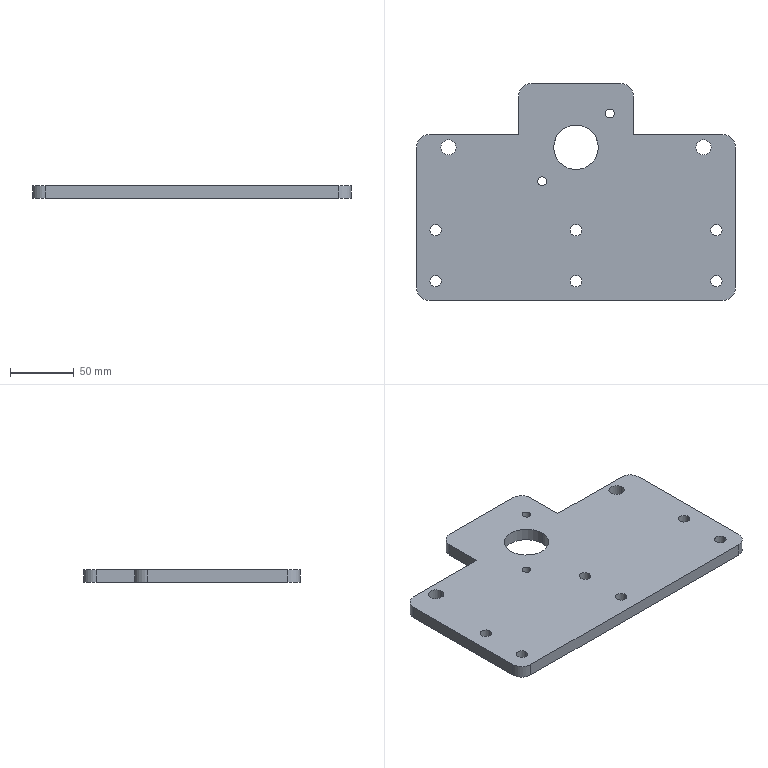Part | SolidWorks | features HoleWzd 3, ICE 2, Extrusion 1, Fillet 1, LPattern 1, MirrorPattern 1 | 1 solid | 38 faces | box 250 x 170 x 10 mm | volume 343286 mm3 | cylinder 28 | plane 10 | commonest cylinder face diameters 9 x12 20 x6 6.8 x4 12 x4 35 x2
STEP:
#1=CARTESIAN_POINT('',(-29.915,8.485,-5.));
#2=VERTEX_POINT('',#1);
#3=CARTESIAN_POINT('',(-23.115,8.485,-5.));
#4=VERTEX_POINT('',#3);
#5=CARTESIAN_POINT('',(-26.515,8.485,-5.));
#6=DIRECTION('',(0.,0.,1.));
#7=DIRECTION('',(1.,0.,0.));
#8=AXIS2_PLACEMENT_3D('',#5,#6,#7);
#9=CIRCLE('',#8,3.4);
#10=EDGE_CURVE('',#2,#4,#9,.T.);
#11=ORIENTED_EDGE('',*,*,#10,.F.);
#12=CARTESIAN_POINT('',(-29.915,8.485,5.));
#13=VERTEX_POINT('',#12);
#14=CARTESIAN_POINT('',(-29.915,8.485,5.));
#15=DIRECTION('',(0.,0.,1.));
#16=VECTOR('',#15,1000.);
#17=LINE('',#14,#16);
#18=EDGE_CURVE('',#2,#13,#17,.T.);
#19=ORIENTED_EDGE('',*,*,#18,.T.);
#20=CARTESIAN_POINT('',(-23.115,8.485,5.));
#21=VERTEX_POINT('',#20);
#22=CARTESIAN_POINT('',(-26.515,8.485,5.));
#23=DIRECTION('',(0.,0.,1.));
#24=DIRECTION('',(1.,0.,0.));
#25=AXIS2_PLACEMENT_3D('',#22,#23,#24);
#26=CIRCLE('',#25,3.4);
#27=EDGE_CURVE('',#13,#21,#26,.T.);
#28=ORIENTED_EDGE('',*,*,#27,.T.);
#29=CARTESIAN_POINT('',(-23.115,8.485,5.));
#30=DIRECTION('',(0.,0.,1.));
#31=VECTOR('',#30,1000.);
#32=LINE('',#29,#31);
#33=EDGE_CURVE('',#4,#21,#32,.T.);
#34=ORIENTED_EDGE('',*,*,#33,.F.);
#35=EDGE_LOOP('',(#11,#19,#28,#34));
#36=FACE_OUTER_BOUND('',#35,.T.);
#37=CARTESIAN_POINT('',(-26.515,8.485,5.));
#38=DIRECTION('',(0.,0.,1.));
#39=DIRECTION('',(1.,0.,0.));
#40=AXIS2_PLACEMENT_3D('',#37,#38,#39);
#41=CYLINDRICAL_SURFACE('',#40,3.4);
#42=ADVANCED_FACE('',(#36),#41,.F.);
#43=CARTESIAN_POINT('',(23.115,61.515,-5.));
#44=VERTEX_POINT('',#43);
#45=CARTESIAN_POINT('',(29.915,61.515,-5.));
#46=VERTEX_POINT('',#45);
#47=CARTESIAN_POINT('',(26.515,61.515,-5.));
#48=DIRECTION('',(0.,0.,1.));
#49=DIRECTION('',(1.,0.,0.));
#50=AXIS2_PLACEMENT_3D('',#47,#48,#49);
#51=CIRCLE('',#50,3.4);
#52=EDGE_CURVE('',#44,#46,#51,.T.);
#53=ORIENTED_EDGE('',*,*,#52,.F.);
#54=CARTESIAN_POINT('',(23.115,61.515,5.));
#55=VERTEX_POINT('',#54);
#56=CARTESIAN_POINT('',(23.115,61.515,5.));
#57=DIRECTION('',(0.,0.,1.));
#58=VECTOR('',#57,1000.);
#59=LINE('',#56,#58);
#60=EDGE_CURVE('',#44,#55,#59,.T.);
#61=ORIENTED_EDGE('',*,*,#60,.T.);
#62=CARTESIAN_POINT('',(29.915,61.515,5.));
#63=VERTEX_POINT('',#62);
#64=CARTESIAN_POINT('',(26.515,61.515,5.));
#65=DIRECTION('',(0.,0.,1.));
#66=DIRECTION('',(1.,0.,0.));
#67=AXIS2_PLACEMENT_3D('',#64,#65,#66);
#68=CIRCLE('',#67,3.4);
#69=EDGE_CURVE('',#55,#63,#68,.T.);
#70=ORIENTED_EDGE('',*,*,#69,.T.);
#71=CARTESIAN_POINT('',(29.915,61.515,5.));
#72=DIRECTION('',(0.,0.,1.));
#73=VECTOR('',#72,1000.);
#74=LINE('',#71,#73);
#75=EDGE_CURVE('',#46,#63,#74,.T.);
#76=ORIENTED_EDGE('',*,*,#75,.F.);
#77=EDGE_LOOP('',(#53,#61,#70,#76));
#78=FACE_OUTER_BOUND('',#77,.T.);
#79=CARTESIAN_POINT('',(26.515,61.515,5.));
#80=DIRECTION('',(0.,0.,1.));
#81=DIRECTION('',(1.,0.,0.));
#82=AXIS2_PLACEMENT_3D('',#79,#80,#81);
#83=CYLINDRICAL_SURFACE('',#82,3.4);
#84=ADVANCED_FACE('',(#78),#83,.F.);
#85=CARTESIAN_POINT('',(-17.5,35.,-5.));
#86=VERTEX_POINT('',#85);
#87=CARTESIAN_POINT('',(17.5,35.,-5.));
#88=VERTEX_POINT('',#87);
#89=CARTESIAN_POINT('',(0.,35.,-5.));
#90=DIRECTION('',(0.,0.,1.));
#91=DIRECTION('',(1.,0.,0.));
#92=AXIS2_PLACEMENT_3D('',#89,#90,#91);
#93=CIRCLE('',#92,17.5);
#94=EDGE_CURVE('',#86,#88,#93,.T.);
#95=ORIENTED_EDGE('',*,*,#94,.F.);
#96=CARTESIAN_POINT('',(-17.5,35.,5.));
#97=VERTEX_POINT('',#96);
#98=CARTESIAN_POINT('',(-17.5,35.,-5.));
#99=DIRECTION('',(0.,0.,1.));
#100=VECTOR('',#99,1000.);
#101=LINE('',#98,#100);
#102=EDGE_CURVE('',#86,#97,#101,.T.);
#103=ORIENTED_EDGE('',*,*,#102,.T.);
#104=CARTESIAN_POINT('',(17.5,35.,5.));
#105=VERTEX_POINT('',#104);
#106=CARTESIAN_POINT('',(0.,35.,5.));
#107=DIRECTION('',(0.,0.,1.));
#108=DIRECTION('',(1.,0.,0.));
#109=AXIS2_PLACEMENT_3D('',#106,#107,#108);
#110=CIRCLE('',#109,17.5);
#111=EDGE_CURVE('',#97,#105,#110,.T.);
#112=ORIENTED_EDGE('',*,*,#111,.T.);
#113=CARTESIAN_POINT('',(17.5,35.,-5.));
#114=DIRECTION('',(0.,0.,1.));
#115=VECTOR('',#114,1000.);
#116=LINE('',#113,#115);
#117=EDGE_CURVE('',#88,#105,#116,.T.);
#118=ORIENTED_EDGE('',*,*,#117,.F.);
#119=EDGE_LOOP('',(#95,#103,#112,#118));
#120=FACE_OUTER_BOUND('',#119,.T.);
#121=CARTESIAN_POINT('',(0.,35.,-5.));
#122=DIRECTION('',(0.,0.,1.));
#123=DIRECTION('',(1.,0.,0.));
#124=AXIS2_PLACEMENT_3D('',#121,#122,#123);
#125=CYLINDRICAL_SURFACE('',#124,17.5);
#126=ADVANCED_FACE('',(#120),#125,.F.);
#127=CARTESIAN_POINT('',(-106.,35.,-5.));
#128=VERTEX_POINT('',#127);
#129=CARTESIAN_POINT('',(-94.,35.,-5.));
#130=VERTEX_POINT('',#129);
#131=CARTESIAN_POINT('',(-100.,35.,-5.));
#132=DIRECTION('',(0.,0.,1.));
#133=DIRECTION('',(1.,0.,0.));
#134=AXIS2_PLACEMENT_3D('',#131,#132,#133);
#135=CIRCLE('',#134,6.);
#136=EDGE_CURVE('',#128,#130,#135,.T.);
#137=ORIENTED_EDGE('',*,*,#136,.F.);
#138=CARTESIAN_POINT('',(-106.,35.,5.));
#139=VERTEX_POINT('',#138);
#140=CARTESIAN_POINT('',(-106.,35.,5.));
#141=DIRECTION('',(0.,0.,1.));
#142=VECTOR('',#141,1000.);
#143=LINE('',#140,#142);
#144=EDGE_CURVE('',#128,#139,#143,.T.);
#145=ORIENTED_EDGE('',*,*,#144,.T.);
#146=CARTESIAN_POINT('',(-94.,35.,5.));
#147=VERTEX_POINT('',#146);
#148=CARTESIAN_POINT('',(-100.,35.,5.));
#149=DIRECTION('',(0.,0.,1.));
#150=DIRECTION('',(1.,0.,0.));
#151=AXIS2_PLACEMENT_3D('',#148,#149,#150);
#152=CIRCLE('',#151,6.);
#153=EDGE_CURVE('',#139,#147,#152,.T.);
#154=ORIENTED_EDGE('',*,*,#153,.T.);
#155=CARTESIAN_POINT('',(-94.,35.,5.));
#156=DIRECTION('',(0.,0.,1.));
#157=VECTOR('',#156,1000.);
#158=LINE('',#155,#157);
#159=EDGE_CURVE('',#130,#147,#158,.T.);
#160=ORIENTED_EDGE('',*,*,#159,.F.);
#161=EDGE_LOOP('',(#137,#145,#154,#160));
#162=FACE_OUTER_BOUND('',#161,.T.);
#163=CARTESIAN_POINT('',(-100.,35.,5.));
#164=DIRECTION('',(0.,0.,1.));
#165=DIRECTION('',(1.,0.,0.));
#166=AXIS2_PLACEMENT_3D('',#163,#164,#165);
#167=CYLINDRICAL_SURFACE('',#166,6.);
#168=ADVANCED_FACE('',(#162),#167,.F.);
#169=CARTESIAN_POINT('',(94.,35.,-5.));
#170=VERTEX_POINT('',#169);
#171=CARTESIAN_POINT('',(106.,35.,-5.));
#172=VERTEX_POINT('',#171);
#173=CARTESIAN_POINT('',(100.,35.,-5.));
#174=DIRECTION('',(0.,0.,1.));
#175=DIRECTION('',(1.,0.,0.));
#176=AXIS2_PLACEMENT_3D('',#173,#174,#175);
#177=CIRCLE('',#176,6.);
#178=EDGE_CURVE('',#170,#172,#177,.T.);
#179=ORIENTED_EDGE('',*,*,#178,.F.);
#180=CARTESIAN_POINT('',(94.,35.,5.));
#181=VERTEX_POINT('',#180);
#182=CARTESIAN_POINT('',(94.,35.,5.));
#183=DIRECTION('',(0.,0.,1.));
#184=VECTOR('',#183,1000.);
#185=LINE('',#182,#184);
#186=EDGE_CURVE('',#170,#181,#185,.T.);
#187=ORIENTED_EDGE('',*,*,#186,.T.);
#188=CARTESIAN_POINT('',(106.,35.,5.));
#189=VERTEX_POINT('',#188);
#190=CARTESIAN_POINT('',(100.,35.,5.));
#191=DIRECTION('',(0.,0.,1.));
#192=DIRECTION('',(1.,0.,0.));
#193=AXIS2_PLACEMENT_3D('',#190,#191,#192);
#194=CIRCLE('',#193,6.);
#195=EDGE_CURVE('',#181,#189,#194,.T.);
#196=ORIENTED_EDGE('',*,*,#195,.T.);
#197=CARTESIAN_POINT('',(106.,35.,5.));
#198=DIRECTION('',(0.,0.,1.));
#199=VECTOR('',#198,1000.);
#200=LINE('',#197,#199);
#201=EDGE_CURVE('',#172,#189,#200,.T.);
#202=ORIENTED_EDGE('',*,*,#201,.F.);
#203=EDGE_LOOP('',(#179,#187,#196,#202));
#204=FACE_OUTER_BOUND('',#203,.T.);
#205=CARTESIAN_POINT('',(100.,35.,5.));
#206=DIRECTION('',(0.,0.,1.));
#207=DIRECTION('',(1.,0.,0.));
#208=AXIS2_PLACEMENT_3D('',#205,#206,#207);
#209=CYLINDRICAL_SURFACE('',#208,6.);
#210=ADVANCED_FACE('',(#204),#209,.F.);
#211=CARTESIAN_POINT('',(105.5,-70.,-5.));
#212=VERTEX_POINT('',#211);
#213=CARTESIAN_POINT('',(114.5,-70.,-5.));
#214=VERTEX_POINT('',#213);
#215=CARTESIAN_POINT('',(110.,-70.,-5.));
#216=DIRECTION('',(0.,0.,1.));
#217=DIRECTION('',(1.,0.,0.));
#218=AXIS2_PLACEMENT_3D('',#215,#216,#217);
#219=CIRCLE('',#218,4.5);
#220=EDGE_CURVE('',#212,#214,#219,.T.);
#221=ORIENTED_EDGE('',*,*,#220,.F.);
#222=CARTESIAN_POINT('',(105.5,-70.,5.));
#223=VERTEX_POINT('',#222);
#224=CARTESIAN_POINT('',(105.5,-70.,5.));
#225=DIRECTION('',(0.,0.,1.));
#226=VECTOR('',#225,1000.);
#227=LINE('',#224,#226);
#228=EDGE_CURVE('',#212,#223,#227,.T.);
#229=ORIENTED_EDGE('',*,*,#228,.T.);
#230=CARTESIAN_POINT('',(114.5,-70.,5.));
#231=VERTEX_POINT('',#230);
#232=CARTESIAN_POINT('',(110.,-70.,5.));
#233=DIRECTION('',(0.,0.,1.));
#234=DIRECTION('',(1.,0.,0.));
#235=AXIS2_PLACEMENT_3D('',#232,#233,#234);
#236=CIRCLE('',#235,4.5);
#237=EDGE_CURVE('',#223,#231,#236,.T.);
#238=ORIENTED_EDGE('',*,*,#237,.T.);
#239=CARTESIAN_POINT('',(114.5,-70.,5.));
#240=DIRECTION('',(0.,0.,1.));
#241=VECTOR('',#240,1000.);
#242=LINE('',#239,#241);
#243=EDGE_CURVE('',#214,#231,#242,.T.);
#244=ORIENTED_EDGE('',*,*,#243,.F.);
#245=EDGE_LOOP('',(#221,#229,#238,#244));
#246=FACE_OUTER_BOUND('',#245,.T.);
#247=CARTESIAN_POINT('',(110.,-70.,5.));
#248=DIRECTION('',(0.,0.,1.));
#249=DIRECTION('',(1.,0.,0.));
#250=AXIS2_PLACEMENT_3D('',#247,#248,#249);
#251=CYLINDRICAL_SURFACE('',#250,4.5);
#252=ADVANCED_FACE('',(#246),#251,.F.);
#253=CARTESIAN_POINT('',(-4.5,-70.,-5.));
#254=VERTEX_POINT('',#253);
#255=CARTESIAN_POINT('',(4.5,-70.,-5.));
#256=VERTEX_POINT('',#255);
#257=CARTESIAN_POINT('',(0.,-70.,-5.));
#258=DIRECTION('',(0.,0.,1.));
#259=DIRECTION('',(1.,0.,0.));
#260=AXIS2_PLACEMENT_3D('',#257,#258,#259);
#261=CIRCLE('',#260,4.5);
#262=EDGE_CURVE('',#254,#256,#261,.T.);
#263=ORIENTED_EDGE('',*,*,#262,.F.);
#264=CARTESIAN_POINT('',(-4.5,-70.,5.));
#265=VERTEX_POINT('',#264);
#266=CARTESIAN_POINT('',(-4.5,-70.,5.));
#267=DIRECTION('',(0.,0.,1.));
#268=VECTOR('',#267,1000.);
#269=LINE('',#266,#268);
#270=EDGE_CURVE('',#254,#265,#269,.T.);
#271=ORIENTED_EDGE('',*,*,#270,.T.);
#272=CARTESIAN_POINT('',(4.5,-70.,5.));
#273=VERTEX_POINT('',#272);
#274=CARTESIAN_POINT('',(0.,-70.,5.));
#275=DIRECTION('',(0.,0.,1.));
#276=DIRECTION('',(1.,0.,0.));
#277=AXIS2_PLACEMENT_3D('',#274,#275,#276);
#278=CIRCLE('',#277,4.5);
#279=EDGE_CURVE('',#265,#273,#278,.T.);
#280=ORIENTED_EDGE('',*,*,#279,.T.);
#281=CARTESIAN_POINT('',(4.5,-70.,5.));
#282=DIRECTION('',(0.,0.,1.));
#283=VECTOR('',#282,1000.);
#284=LINE('',#281,#283);
#285=EDGE_CURVE('',#256,#273,#284,.T.);
#286=ORIENTED_EDGE('',*,*,#285,.F.);
#287=EDGE_LOOP('',(#263,#271,#280,#286));
#288=FACE_OUTER_BOUND('',#287,.T.);
#289=CARTESIAN_POINT('',(0.,-70.,5.));
#290=DIRECTION('',(0.,0.,1.));
#291=DIRECTION('',(1.,0.,0.));
#292=AXIS2_PLACEMENT_3D('',#289,#290,#291);
#293=CYLINDRICAL_SURFACE('',#292,4.5);
#294=ADVANCED_FACE('',(#288),#293,.F.);
#295=CARTESIAN_POINT('',(105.5,-30.,-5.));
#296=VERTEX_POINT('',#295);
#297=CARTESIAN_POINT('',(114.5,-30.,-5.));
#298=VERTEX_POINT('',#297);
#299=CARTESIAN_POINT('',(110.,-30.,-5.));
#300=DIRECTION('',(0.,0.,1.));
#301=DIRECTION('',(1.,0.,0.));
#302=AXIS2_PLACEMENT_3D('',#299,#300,#301);
#303=CIRCLE('',#302,4.5);
#304=EDGE_CURVE('',#296,#298,#303,.T.);
#305=ORIENTED_EDGE('',*,*,#304,.F.);
#306=CARTESIAN_POINT('',(105.5,-30.,5.));
#307=VERTEX_POINT('',#306);
#308=CARTESIAN_POINT('',(105.5,-30.,5.));
#309=DIRECTION('',(0.,0.,1.));
#310=VECTOR('',#309,1000.);
#311=LINE('',#308,#310);
#312=EDGE_CURVE('',#296,#307,#311,.T.);
#313=ORIENTED_EDGE('',*,*,#312,.T.);
#314=CARTESIAN_POINT('',(114.5,-30.,5.));
#315=VERTEX_POINT('',#314);
#316=CARTESIAN_POINT('',(110.,-30.,5.));
#317=DIRECTION('',(0.,0.,1.));
#318=DIRECTION('',(1.,0.,0.));
#319=AXIS2_PLACEMENT_3D('',#316,#317,#318);
#320=CIRCLE('',#319,4.5);
#321=EDGE_CURVE('',#307,#315,#320,.T.);
#322=ORIENTED_EDGE('',*,*,#321,.T.);
#323=CARTESIAN_POINT('',(114.5,-30.,5.));
#324=DIRECTION('',(0.,0.,1.));
#325=VECTOR('',#324,1000.);
#326=LINE('',#323,#325);
#327=EDGE_CURVE('',#298,#315,#326,.T.);
#328=ORIENTED_EDGE('',*,*,#327,.F.);
#329=EDGE_LOOP('',(#305,#313,#322,#328));
#330=FACE_OUTER_BOUND('',#329,.T.);
#331=CARTESIAN_POINT('',(110.,-30.,5.));
#332=DIRECTION('',(0.,0.,1.));
#333=DIRECTION('',(1.,0.,0.));
#334=AXIS2_PLACEMENT_3D('',#331,#332,#333);
#335=CYLINDRICAL_SURFACE('',#334,4.5);
#336=ADVANCED_FACE('',(#330),#335,.F.);
#337=CARTESIAN_POINT('',(-4.5,-30.,-5.));
#338=VERTEX_POINT('',#337);
#339=CARTESIAN_POINT('',(4.5,-30.,-5.));
#340=VERTEX_POINT('',#339);
#341=CARTESIAN_POINT('',(0.,-30.,-5.));
#342=DIRECTION('',(0.,0.,1.));
#343=DIRECTION('',(1.,0.,0.));
#344=AXIS2_PLACEMENT_3D('',#341,#342,#343);
#345=CIRCLE('',#344,4.5);
#346=EDGE_CURVE('',#338,#340,#345,.T.);
#347=ORIENTED_EDGE('',*,*,#346,.F.);
#348=CARTESIAN_POINT('',(-4.5,-30.,5.));
#349=VERTEX_POINT('',#348);
#350=CARTESIAN_POINT('',(-4.5,-30.,5.));
#351=DIRECTION('',(0.,0.,1.));
#352=VECTOR('',#351,1000.);
#353=LINE('',#350,#352);
#354=EDGE_CURVE('',#338,#349,#353,.T.);
#355=ORIENTED_EDGE('',*,*,#354,.T.);
#356=CARTESIAN_POINT('',(4.5,-30.,5.));
#357=VERTEX_POINT('',#356);
#358=CARTESIAN_POINT('',(0.,-30.,5.));
#359=DIRECTION('',(0.,0.,1.));
#360=DIRECTION('',(1.,0.,0.));
#361=AXIS2_PLACEMENT_3D('',#358,#359,#360);
#362=CIRCLE('',#361,4.5);
#363=EDGE_CURVE('',#349,#357,#362,.T.);
#364=ORIENTED_EDGE('',*,*,#363,.T.);
#365=CARTESIAN_POINT('',(4.5,-30.,5.));
#366=DIRECTION('',(0.,0.,1.));
#367=VECTOR('',#366,1000.);
#368=LINE('',#365,#367);
#369=EDGE_CURVE('',#340,#357,#368,.T.);
#370=ORIENTED_EDGE('',*,*,#369,.F.);
#371=EDGE_LOOP('',(#347,#355,#364,#370));
#372=FACE_OUTER_BOUND('',#371,.T.);
#373=CARTESIAN_POINT('',(0.,-30.,5.));
#374=DIRECTION('',(0.,0.,1.));
#375=DIRECTION('',(1.,0.,0.));
#376=AXIS2_PLACEMENT_3D('',#373,#374,#375);
#377=CYLINDRICAL_SURFACE('',#376,4.5);
#378=ADVANCED_FACE('',(#372),#377,.F.);
#379=CARTESIAN_POINT('',(-114.5,-30.,-5.));
#380=VERTEX_POINT('',#379);
#381=CARTESIAN_POINT('',(-105.5,-30.,-5.));
#382=VERTEX_POINT('',#381);
#383=CARTESIAN_POINT('',(-110.,-30.,-5.));
#384=DIRECTION('',(0.,0.,1.));
#385=DIRECTION('',(1.,0.,0.));
#386=AXIS2_PLACEMENT_3D('',#383,#384,#385);
#387=CIRCLE('',#386,4.5);
#388=EDGE_CURVE('',#380,#382,#387,.T.);
#389=ORIENTED_EDGE('',*,*,#388,.F.);
#390=CARTESIAN_POINT('',(-114.5,-30.,5.));
#391=VERTEX_POINT('',#390);
#392=CARTESIAN_POINT('',(-114.5,-30.,5.));
#393=DIRECTION('',(0.,0.,1.));
#394=VECTOR('',#393,1000.);
#395=LINE('',#392,#394);
#396=EDGE_CURVE('',#380,#391,#395,.T.);
#397=ORIENTED_EDGE('',*,*,#396,.T.);
#398=CARTESIAN_POINT('',(-105.5,-30.,5.));
#399=VERTEX_POINT('',#398);
#400=CARTESIAN_POINT('',(-110.,-30.,5.));
#401=DIRECTION('',(0.,0.,1.));
#402=DIRECTION('',(1.,0.,0.));
#403=AXIS2_PLACEMENT_3D('',#400,#401,#402);
#404=CIRCLE('',#403,4.5);
#405=EDGE_CURVE('',#391,#399,#404,.T.);
#406=ORIENTED_EDGE('',*,*,#405,.T.);
#407=CARTESIAN_POINT('',(-105.5,-30.,5.));
#408=DIRECTION('',(0.,0.,1.));
#409=VECTOR('',#408,1000.);
#410=LINE('',#407,#409);
#411=EDGE_CURVE('',#382,#399,#410,.T.);
#412=ORIENTED_EDGE('',*,*,#411,.F.);
#413=EDGE_LOOP('',(#389,#397,#406,#412));
#414=FACE_OUTER_BOUND('',#413,.T.);
#415=CARTESIAN_POINT('',(-110.,-30.,5.));
#416=DIRECTION('',(0.,0.,1.));
#417=DIRECTION('',(1.,0.,0.));
#418=AXIS2_PLACEMENT_3D('',#415,#416,#417);
#419=CYLINDRICAL_SURFACE('',#418,4.5);
#420=ADVANCED_FACE('',(#414),#419,.F.);
#421=CARTESIAN_POINT('',(-114.5,-70.,-5.));
#422=VERTEX_POINT('',#421);
#423=CARTESIAN_POINT('',(-105.5,-70.,-5.));
#424=VERTEX_POINT('',#423);
#425=CARTESIAN_POINT('',(-110.,-70.,-5.));
#426=DIRECTION('',(0.,0.,1.));
#427=DIRECTION('',(1.,0.,0.));
#428=AXIS2_PLACEMENT_3D('',#425,#426,#427);
#429=CIRCLE('',#428,4.5);
#430=EDGE_CURVE('',#422,#424,#429,.T.);
#431=ORIENTED_EDGE('',*,*,#430,.F.);
#432=CARTESIAN_POINT('',(-114.5,-70.,5.));
#433=VERTEX_POINT('',#432);
#434=CARTESIAN_POINT('',(-114.5,-70.,5.));
#435=DIRECTION('',(0.,0.,1.));
#436=VECTOR('',#435,1000.);
#437=LINE('',#434,#436);
#438=EDGE_CURVE('',#422,#433,#437,.T.);
#439=ORIENTED_EDGE('',*,*,#438,.T.);
#440=CARTESIAN_POINT('',(-105.5,-70.,5.));
#441=VERTEX_POINT('',#440);
#442=CARTESIAN_POINT('',(-110.,-70.,5.));
#443=DIRECTION('',(0.,0.,1.));
#444=DIRECTION('',(1.,0.,0.));
#445=AXIS2_PLACEMENT_3D('',#442,#443,#444);
#446=CIRCLE('',#445,4.5);
#447=EDGE_CURVE('',#433,#441,#446,.T.);
#448=ORIENTED_EDGE('',*,*,#447,.T.);
#449=CARTESIAN_POINT('',(-105.5,-70.,5.));
#450=DIRECTION('',(0.,0.,1.));
#451=VECTOR('',#450,1000.);
#452=LINE('',#449,#451);
#453=EDGE_CURVE('',#424,#441,#452,.T.);
#454=ORIENTED_EDGE('',*,*,#453,.F.);
#455=EDGE_LOOP('',(#431,#439,#448,#454));
#456=FACE_OUTER_BOUND('',#455,.T.);
#457=CARTESIAN_POINT('',(-110.,-70.,5.));
#458=DIRECTION('',(0.,0.,1.));
#459=DIRECTION('',(1.,0.,0.));
#460=AXIS2_PLACEMENT_3D('',#457,#458,#459);
#461=CYLINDRICAL_SURFACE('',#460,4.5);
#462=ADVANCED_FACE('',(#456),#461,.F.);
#463=CARTESIAN_POINT('',(35.,85.,5.));
#464=VERTEX_POINT('',#463);
#465=CARTESIAN_POINT('',(-35.,85.,5.));
#466=VERTEX_POINT('',#465);
#467=CARTESIAN_POINT('',(-125.,85.,5.));
#468=DIRECTION('',(-1.,0.,0.));
#469=VECTOR('',#468,1000.);
#470=LINE('',#467,#469);
#471=EDGE_CURVE('',#464,#466,#470,.T.);
#472=ORIENTED_EDGE('',*,*,#471,.F.);
#473=CARTESIAN_POINT('',(35.,85.,-5.));
#474=VERTEX_POINT('',#473);
#475=CARTESIAN_POINT('',(35.,85.,5.));
#476=DIRECTION('',(0.,0.,-1.));
#477=VECTOR('',#476,1000.);
#478=LINE('',#475,#477);
#479=EDGE_CURVE('',#464,#474,#478,.T.);
#480=ORIENTED_EDGE('',*,*,#479,.T.);
#481=CARTESIAN_POINT('',(-35.,85.,-5.));
#482=VERTEX_POINT('',#481);
#483=CARTESIAN_POINT('',(-125.,85.,-5.));
#484=DIRECTION('',(-1.,0.,0.));
#485=VECTOR('',#484,1000.);
#486=LINE('',#483,#485);
#487=EDGE_CURVE('',#474,#482,#486,.T.);
#488=ORIENTED_EDGE('',*,*,#487,.T.);
#489=CARTESIAN_POINT('',(-35.,85.,5.));
#490=DIRECTION('',(0.,0.,1.));
#491=VECTOR('',#490,1000.);
#492=LINE('',#489,#491);
#493=EDGE_CURVE('',#482,#466,#492,.T.);
#494=ORIENTED_EDGE('',*,*,#493,.T.);
#495=EDGE_LOOP('',(#472,#480,#488,#494));
#496=FACE_OUTER_BOUND('',#495,.T.);
#497=CARTESIAN_POINT('',(-125.,85.,5.));
#498=DIRECTION('',(0.,-1.,0.));
#499=DIRECTION('',(0.,0.,-1.));
#500=AXIS2_PLACEMENT_3D('',#497,#498,#499);
#501=PLANE('',#500);
#502=ADVANCED_FACE('',(#496),#501,.F.);
#503=CARTESIAN_POINT('',(-125.,35.,-5.));
#504=VERTEX_POINT('',#503);
#505=CARTESIAN_POINT('',(-125.,-75.,-5.));
#506=VERTEX_POINT('',#505);
#507=CARTESIAN_POINT('',(-125.,85.,-5.));
#508=DIRECTION('',(0.,-1.,0.));
#509=VECTOR('',#508,1000.);
#510=LINE('',#507,#509);
#511=EDGE_CURVE('',#504,#506,#510,.T.);
#512=ORIENTED_EDGE('',*,*,#511,.T.);
#513=CARTESIAN_POINT('',(-125.,-75.,5.));
#514=VERTEX_POINT('',#513);
#515=CARTESIAN_POINT('',(-125.,-75.,5.));
#516=DIRECTION('',(0.,0.,1.));
#517=VECTOR('',#516,1000.);
#518=LINE('',#515,#517);
#519=EDGE_CURVE('',#506,#514,#518,.T.);
#520=ORIENTED_EDGE('',*,*,#519,.T.);
#521=CARTESIAN_POINT('',(-125.,35.,5.));
#522=VERTEX_POINT('',#521);
#523=CARTESIAN_POINT('',(-125.,85.,5.));
#524=DIRECTION('',(0.,-1.,0.));
#525=VECTOR('',#524,1000.);
#526=LINE('',#523,#525);
#527=EDGE_CURVE('',#522,#514,#526,.T.);
#528=ORIENTED_EDGE('',*,*,#527,.F.);
#529=CARTESIAN_POINT('',(-125.,35.,-5.));
#530=DIRECTION('',(0.,0.,-1.));
#531=VECTOR('',#530,1000.);
#532=LINE('',#529,#531);
#533=EDGE_CURVE('',#522,#504,#532,.T.);
#534=ORIENTED_EDGE('',*,*,#533,.T.);
#535=EDGE_LOOP('',(#512,#520,#528,#534));
#536=FACE_OUTER_BOUND('',#535,.T.);
#537=CARTESIAN_POINT('',(-125.,85.,5.));
#538=DIRECTION('',(1.,0.,0.));
#539=DIRECTION('',(0.,1.,0.));
#540=AXIS2_PLACEMENT_3D('',#537,#538,#539);
#541=PLANE('',#540);
#542=ADVANCED_FACE('',(#536),#541,.F.);
#543=CARTESIAN_POINT('',(-26.515,8.485,5.));
#544=DIRECTION('',(0.,0.,1.));
#545=DIRECTION('',(1.,0.,0.));
#546=AXIS2_PLACEMENT_3D('',#543,#544,#545);
#547=CIRCLE('',#546,3.4);
#548=EDGE_CURVE('',#21,#13,#547,.T.);
#549=ORIENTED_EDGE('',*,*,#548,.F.);
#550=ORIENTED_EDGE('',*,*,#27,.F.);
#551=EDGE_LOOP('',(#549,#550));
#552=FACE_BOUND('',#551,.T.);
#553=CARTESIAN_POINT('',(26.515,61.515,5.));
#554=DIRECTION('',(0.,0.,1.));
#555=DIRECTION('',(1.,0.,0.));
#556=AXIS2_PLACEMENT_3D('',#553,#554,#555);
#557=CIRCLE('',#556,3.4);
#558=EDGE_CURVE('',#63,#55,#557,.T.);
#559=ORIENTED_EDGE('',*,*,#558,.F.);
#560=ORIENTED_EDGE('',*,*,#69,.F.);
#561=EDGE_LOOP('',(#559,#560));
#562=FACE_BOUND('',#561,.T.);
#563=CARTESIAN_POINT('',(0.,35.,5.));
#564=DIRECTION('',(0.,0.,1.));
#565=DIRECTION('',(1.,0.,0.));
#566=AXIS2_PLACEMENT_3D('',#563,#564,#565);
#567=CIRCLE('',#566,17.5);
#568=EDGE_CURVE('',#105,#97,#567,.T.);
#569=ORIENTED_EDGE('',*,*,#568,.F.);
#570=ORIENTED_EDGE('',*,*,#111,.F.);
#571=EDGE_LOOP('',(#569,#570));
#572=FACE_BOUND('',#571,.T.);
#573=CARTESIAN_POINT('',(-100.,35.,5.));
#574=DIRECTION('',(0.,0.,1.));
#575=DIRECTION('',(1.,0.,0.));
#576=AXIS2_PLACEMENT_3D('',#573,#574,#575);
#577=CIRCLE('',#576,6.);
#578=EDGE_CURVE('',#147,#139,#577,.T.);
#579=ORIENTED_EDGE('',*,*,#578,.F.);
#580=ORIENTED_EDGE('',*,*,#153,.F.);
#581=EDGE_LOOP('',(#579,#580));
#582=FACE_BOUND('',#581,.T.);
#583=CARTESIAN_POINT('',(100.,35.,5.));
#584=DIRECTION('',(0.,0.,1.));
#585=DIRECTION('',(1.,0.,0.));
#586=AXIS2_PLACEMENT_3D('',#583,#584,#585);
#587=CIRCLE('',#586,6.);
#588=EDGE_CURVE('',#189,#181,#587,.T.);
#589=ORIENTED_EDGE('',*,*,#588,.F.);
#590=ORIENTED_EDGE('',*,*,#195,.F.);
#591=EDGE_LOOP('',(#589,#590));
#592=FACE_BOUND('',#591,.T.);
#593=CARTESIAN_POINT('',(0.,-70.,5.));
#594=DIRECTION('',(0.,0.,1.));
#595=DIRECTION('',(1.,0.,0.));
#596=AXIS2_PLACEMENT_3D('',#593,#594,#595);
#597=CIRCLE('',#596,4.5);
#598=EDGE_CURVE('',#273,#265,#597,.T.);
#599=ORIENTED_EDGE('',*,*,#598,.F.);
#600=ORIENTED_EDGE('',*,*,#279,.F.);
#601=EDGE_LOOP('',(#599,#600));
#602=FACE_BOUND('',#601,.T.);
#603=CARTESIAN_POINT('',(0.,-30.,5.));
#604=DIRECTION('',(0.,0.,1.));
#605=DIRECTION('',(1.,0.,0.));
#606=AXIS2_PLACEMENT_3D('',#603,#604,#605);
#607=CIRCLE('',#606,4.5);
#608=EDGE_CURVE('',#357,#349,#607,.T.);
#609=ORIENTED_EDGE('',*,*,#608,.F.);
#610=ORIENTED_EDGE('',*,*,#363,.F.);
#611=EDGE_LOOP('',(#609,#610));
#612=FACE_BOUND('',#611,.T.);
#613=CARTESIAN_POINT('',(-110.,-30.,5.));
#614=DIRECTION('',(0.,0.,1.));
#615=DIRECTION('',(1.,0.,0.));
#616=AXIS2_PLACEMENT_3D('',#613,#614,#615);
#617=CIRCLE('',#616,4.5);
#618=EDGE_CURVE('',#399,#391,#617,.T.);
#619=ORIENTED_EDGE('',*,*,#618,.F.);
#620=ORIENTED_EDGE('',*,*,#405,.F.);
#621=EDGE_LOOP('',(#619,#620));
#622=FACE_BOUND('',#621,.T.);
#623=CARTESIAN_POINT('',(-110.,-70.,5.));
#624=DIRECTION('',(0.,0.,1.));
#625=DIRECTION('',(1.,0.,0.));
#626=AXIS2_PLACEMENT_3D('',#623,#624,#625);
#627=CIRCLE('',#626,4.5);
#628=EDGE_CURVE('',#441,#433,#627,.T.);
#629=ORIENTED_EDGE('',*,*,#628,.F.);
#630=ORIENTED_EDGE('',*,*,#447,.F.);
#631=EDGE_LOOP('',(#629,#630));
#632=FACE_BOUND('',#631,.T.);
#633=CARTESIAN_POINT('',(-115.,-85.,5.));
#634=VERTEX_POINT('',#633);
#635=CARTESIAN_POINT('',(115.,-85.,5.));
#636=VERTEX_POINT('',#635);
#637=CARTESIAN_POINT('',(-125.,-85.,5.));
#638=DIRECTION('',(1.,0.,0.));
#639=VECTOR('',#638,1000.);
#640=LINE('',#637,#639);
#641=EDGE_CURVE('',#634,#636,#640,.T.);
#642=ORIENTED_EDGE('',*,*,#641,.T.);
#643=CARTESIAN_POINT('',(125.,-75.,5.));
#644=VERTEX_POINT('',#643);
#645=CARTESIAN_POINT('',(115.,-75.,5.));
#646=DIRECTION('',(0.,0.,1.));
#647=DIRECTION('',(1.,0.,0.));
#648=AXIS2_PLACEMENT_3D('',#645,#646,#647);
#649=CIRCLE('',#648,10.);
#650=EDGE_CURVE('',#636,#644,#649,.T.);
#651=ORIENTED_EDGE('',*,*,#650,.T.);
#652=CARTESIAN_POINT('',(125.,35.,5.));
#653=VERTEX_POINT('',#652);
#654=CARTESIAN_POINT('',(125.,85.,5.));
#655=DIRECTION('',(0.,1.,0.));
#656=VECTOR('',#655,1000.);
#657=LINE('',#654,#656);
#658=EDGE_CURVE('',#644,#653,#657,.T.);
#659=ORIENTED_EDGE('',*,*,#658,.T.);
#660=CARTESIAN_POINT('',(115.,45.,5.));
#661=VERTEX_POINT('',#660);
#662=CARTESIAN_POINT('',(115.,35.,5.));
#663=DIRECTION('',(0.,0.,1.));
#664=DIRECTION('',(1.,0.,0.));
#665=AXIS2_PLACEMENT_3D('',#662,#663,#664);
#666=CIRCLE('',#665,10.);
#667=EDGE_CURVE('',#653,#661,#666,.T.);
#668=ORIENTED_EDGE('',*,*,#667,.T.);
#669=CARTESIAN_POINT('',(45.,45.,5.));
#670=VERTEX_POINT('',#669);
#671=CARTESIAN_POINT('',(45.,45.,5.));
#672=DIRECTION('',(1.,0.,0.));
#673=VECTOR('',#672,1000.);
#674=LINE('',#671,#673);
#675=EDGE_CURVE('',#670,#661,#674,.T.);
#676=ORIENTED_EDGE('',*,*,#675,.F.);
#677=CARTESIAN_POINT('',(45.,75.,5.));
#678=VERTEX_POINT('',#677);
#679=CARTESIAN_POINT('',(45.,85.,5.));
#680=DIRECTION('',(0.,-1.,0.));
#681=VECTOR('',#680,1000.);
#682=LINE('',#679,#681);
#683=EDGE_CURVE('',#678,#670,#682,.T.);
#684=ORIENTED_EDGE('',*,*,#683,.F.);
#685=CARTESIAN_POINT('',(35.,75.,5.));
#686=DIRECTION('',(0.,0.,1.));
#687=DIRECTION('',(1.,0.,0.));
#688=AXIS2_PLACEMENT_3D('',#685,#686,#687);
#689=CIRCLE('',#688,10.);
#690=EDGE_CURVE('',#678,#464,#689,.T.);
#691=ORIENTED_EDGE('',*,*,#690,.T.);
#692=ORIENTED_EDGE('',*,*,#471,.T.);
#693=CARTESIAN_POINT('',(-45.,75.,5.));
#694=VERTEX_POINT('',#693);
#695=CARTESIAN_POINT('',(-35.,75.,5.));
#696=DIRECTION('',(0.,0.,1.));
#697=DIRECTION('',(1.,0.,0.));
#698=AXIS2_PLACEMENT_3D('',#695,#696,#697);
#699=CIRCLE('',#698,10.);
#700=EDGE_CURVE('',#466,#694,#699,.T.);
#701=ORIENTED_EDGE('',*,*,#700,.T.);
#702=CARTESIAN_POINT('',(-45.,45.,5.));
#703=VERTEX_POINT('',#702);
#704=CARTESIAN_POINT('',(-45.,85.,5.));
#705=DIRECTION('',(0.,-1.,0.));
#706=VECTOR('',#705,1000.);
#707=LINE('',#704,#706);
#708=EDGE_CURVE('',#694,#703,#707,.T.);
#709=ORIENTED_EDGE('',*,*,#708,.T.);
#710=CARTESIAN_POINT('',(-115.,45.,5.));
#711=VERTEX_POINT('',#710);
#712=CARTESIAN_POINT('',(-45.,45.,5.));
#713=DIRECTION('',(-1.,0.,0.));
#714=VECTOR('',#713,1000.);
#715=LINE('',#712,#714);
#716=EDGE_CURVE('',#703,#711,#715,.T.);
#717=ORIENTED_EDGE('',*,*,#716,.T.);
#718=CARTESIAN_POINT('',(-115.,35.,5.));
#719=DIRECTION('',(0.,0.,1.));
#720=DIRECTION('',(1.,0.,0.));
#721=AXIS2_PLACEMENT_3D('',#718,#719,#720);
#722=CIRCLE('',#721,10.);
#723=EDGE_CURVE('',#711,#522,#722,.T.);
#724=ORIENTED_EDGE('',*,*,#723,.T.);
#725=ORIENTED_EDGE('',*,*,#527,.T.);
#726=CARTESIAN_POINT('',(-115.,-75.,5.));
#727=DIRECTION('',(0.,0.,1.));
#728=DIRECTION('',(1.,0.,0.));
#729=AXIS2_PLACEMENT_3D('',#726,#727,#728);
#730=CIRCLE('',#729,10.);
#731=EDGE_CURVE('',#514,#634,#730,.T.);
#732=ORIENTED_EDGE('',*,*,#731,.T.);
#733=EDGE_LOOP('',(#642,#651,#659,#668,#676,#684,#691,#692,#701,#709,#717,#724,#725,#732));
#734=FACE_OUTER_BOUND('',#733,.T.);
#735=CARTESIAN_POINT('',(110.,-30.,5.));
#736=DIRECTION('',(0.,0.,1.));
#737=DIRECTION('',(1.,0.,0.));
#738=AXIS2_PLACEMENT_3D('',#735,#736,#737);
#739=CIRCLE('',#738,4.5);
#740=EDGE_CURVE('',#315,#307,#739,.T.);
#741=ORIENTED_EDGE('',*,*,#740,.F.);
#742=ORIENTED_EDGE('',*,*,#321,.F.);
#743=EDGE_LOOP('',(#741,#742));
#744=FACE_BOUND('',#743,.T.);
#745=CARTESIAN_POINT('',(110.,-70.,5.));
#746=DIRECTION('',(0.,0.,1.));
#747=DIRECTION('',(1.,0.,0.));
#748=AXIS2_PLACEMENT_3D('',#745,#746,#747);
#749=CIRCLE('',#748,4.5);
#750=EDGE_CURVE('',#231,#223,#749,.T.);
#751=ORIENTED_EDGE('',*,*,#750,.F.);
#752=ORIENTED_EDGE('',*,*,#237,.F.);
#753=EDGE_LOOP('',(#751,#752));
#754=FACE_BOUND('',#753,.T.);
#755=CARTESIAN_POINT('',(0.,0.,5.));
#756=DIRECTION('',(0.,0.,1.));
#757=DIRECTION('',(1.,0.,0.));
#758=AXIS2_PLACEMENT_3D('',#755,#756,#757);
#759=PLANE('',#758);
#760=ADVANCED_FACE('',(#552,#562,#572,#582,#592,#602,#612,#622,#632,#734,#744,#754),#759,.T.);
#761=CARTESIAN_POINT('',(-26.515,8.485,-5.));
#762=DIRECTION('',(0.,0.,1.));
#763=DIRECTION('',(1.,0.,0.));
#764=AXIS2_PLACEMENT_3D('',#761,#762,#763);
#765=CIRCLE('',#764,3.4);
#766=EDGE_CURVE('',#4,#2,#765,.T.);
#767=ORIENTED_EDGE('',*,*,#766,.T.);
#768=ORIENTED_EDGE('',*,*,#10,.T.);
#769=EDGE_LOOP('',(#767,#768));
#770=FACE_BOUND('',#769,.T.);
#771=CARTESIAN_POINT('',(26.515,61.515,-5.));
#772=DIRECTION('',(0.,0.,1.));
#773=DIRECTION('',(1.,0.,0.));
#774=AXIS2_PLACEMENT_3D('',#771,#772,#773);
#775=CIRCLE('',#774,3.4);
#776=EDGE_CURVE('',#46,#44,#775,.T.);
#777=ORIENTED_EDGE('',*,*,#776,.T.);
#778=ORIENTED_EDGE('',*,*,#52,.T.);
#779=EDGE_LOOP('',(#777,#778));
#780=FACE_BOUND('',#779,.T.);
#781=CARTESIAN_POINT('',(0.,35.,-5.));
#782=DIRECTION('',(0.,0.,1.));
#783=DIRECTION('',(1.,0.,0.));
#784=AXIS2_PLACEMENT_3D('',#781,#782,#783);
#785=CIRCLE('',#784,17.5);
#786=EDGE_CURVE('',#88,#86,#785,.T.);
#787=ORIENTED_EDGE('',*,*,#786,.T.);
#788=ORIENTED_EDGE('',*,*,#94,.T.);
#789=EDGE_LOOP('',(#787,#788));
#790=FACE_BOUND('',#789,.T.);
#791=CARTESIAN_POINT('',(-100.,35.,-5.));
#792=DIRECTION('',(0.,0.,1.));
#793=DIRECTION('',(1.,0.,0.));
#794=AXIS2_PLACEMENT_3D('',#791,#792,#793);
#795=CIRCLE('',#794,6.);
#796=EDGE_CURVE('',#130,#128,#795,.T.);
#797=ORIENTED_EDGE('',*,*,#796,.T.);
#798=ORIENTED_EDGE('',*,*,#136,.T.);
#799=EDGE_LOOP('',(#797,#798));
#800=FACE_BOUND('',#799,.T.);
#801=CARTESIAN_POINT('',(100.,35.,-5.));
#802=DIRECTION('',(0.,0.,1.));
#803=DIRECTION('',(1.,0.,0.));
#804=AXIS2_PLACEMENT_3D('',#801,#802,#803);
#805=CIRCLE('',#804,6.);
#806=EDGE_CURVE('',#172,#170,#805,.T.);
#807=ORIENTED_EDGE('',*,*,#806,.T.);
#808=ORIENTED_EDGE('',*,*,#178,.T.);
#809=EDGE_LOOP('',(#807,#808));
#810=FACE_BOUND('',#809,.T.);
#811=CARTESIAN_POINT('',(0.,-70.,-5.));
#812=DIRECTION('',(0.,0.,1.));
#813=DIRECTION('',(1.,0.,0.));
#814=AXIS2_PLACEMENT_3D('',#811,#812,#813);
#815=CIRCLE('',#814,4.5);
#816=EDGE_CURVE('',#256,#254,#815,.T.);
#817=ORIENTED_EDGE('',*,*,#816,.T.);
#818=ORIENTED_EDGE('',*,*,#262,.T.);
#819=EDGE_LOOP('',(#817,#818));
#820=FACE_BOUND('',#819,.T.);
#821=CARTESIAN_POINT('',(0.,-30.,-5.));
#822=DIRECTION('',(0.,0.,1.));
#823=DIRECTION('',(1.,0.,0.));
#824=AXIS2_PLACEMENT_3D('',#821,#822,#823);
#825=CIRCLE('',#824,4.5);
#826=EDGE_CURVE('',#340,#338,#825,.T.);
#827=ORIENTED_EDGE('',*,*,#826,.T.);
#828=ORIENTED_EDGE('',*,*,#346,.T.);
#829=EDGE_LOOP('',(#827,#828));
#830=FACE_BOUND('',#829,.T.);
#831=CARTESIAN_POINT('',(-110.,-30.,-5.));
#832=DIRECTION('',(0.,0.,1.));
#833=DIRECTION('',(1.,0.,0.));
#834=AXIS2_PLACEMENT_3D('',#831,#832,#833);
#835=CIRCLE('',#834,4.5);
#836=EDGE_CURVE('',#382,#380,#835,.T.);
#837=ORIENTED_EDGE('',*,*,#836,.T.);
#838=ORIENTED_EDGE('',*,*,#388,.T.);
#839=EDGE_LOOP('',(#837,#838));
#840=FACE_BOUND('',#839,.T.);
#841=CARTESIAN_POINT('',(-110.,-70.,-5.));
#842=DIRECTION('',(0.,0.,1.));
#843=DIRECTION('',(1.,0.,0.));
#844=AXIS2_PLACEMENT_3D('',#841,#842,#843);
#845=CIRCLE('',#844,4.5);
#846=EDGE_CURVE('',#424,#422,#845,.T.);
#847=ORIENTED_EDGE('',*,*,#846,.T.);
#848=ORIENTED_EDGE('',*,*,#430,.T.);
#849=EDGE_LOOP('',(#847,#848));
#850=FACE_BOUND('',#849,.T.);
#851=CARTESIAN_POINT('',(125.,-75.,-5.));
#852=VERTEX_POINT('',#851);
#853=CARTESIAN_POINT('',(125.,35.,-5.));
#854=VERTEX_POINT('',#853);
#855=CARTESIAN_POINT('',(125.,85.,-5.));
#856=DIRECTION('',(0.,1.,0.));
#857=VECTOR('',#856,1000.);
#858=LINE('',#855,#857);
#859=EDGE_CURVE('',#852,#854,#858,.T.);
#860=ORIENTED_EDGE('',*,*,#859,.F.);
#861=CARTESIAN_POINT('',(115.,-85.,-5.));
#862=VERTEX_POINT('',#861);
#863=CARTESIAN_POINT('',(115.,-75.,-5.));
#864=DIRECTION('',(0.,0.,-1.));
#865=DIRECTION('',(1.,0.,0.));
#866=AXIS2_PLACEMENT_3D('',#863,#864,#865);
#867=CIRCLE('',#866,10.);
#868=EDGE_CURVE('',#852,#862,#867,.T.);
#869=ORIENTED_EDGE('',*,*,#868,.T.);
#870=CARTESIAN_POINT('',(-115.,-85.,-5.));
#871=VERTEX_POINT('',#870);
#872=CARTESIAN_POINT('',(-125.,-85.,-5.));
#873=DIRECTION('',(1.,0.,0.));
#874=VECTOR('',#873,1000.);
#875=LINE('',#872,#874);
#876=EDGE_CURVE('',#871,#862,#875,.T.);
#877=ORIENTED_EDGE('',*,*,#876,.F.);
#878=CARTESIAN_POINT('',(-115.,-75.,-5.));
#879=DIRECTION('',(0.,0.,-1.));
#880=DIRECTION('',(1.,0.,0.));
#881=AXIS2_PLACEMENT_3D('',#878,#879,#880);
#882=CIRCLE('',#881,10.);
#883=EDGE_CURVE('',#871,#506,#882,.T.);
#884=ORIENTED_EDGE('',*,*,#883,.T.);
#885=ORIENTED_EDGE('',*,*,#511,.F.);
#886=CARTESIAN_POINT('',(-115.,45.,-5.));
#887=VERTEX_POINT('',#886);
#888=CARTESIAN_POINT('',(-115.,35.,-5.));
#889=DIRECTION('',(0.,0.,-1.));
#890=DIRECTION('',(1.,0.,0.));
#891=AXIS2_PLACEMENT_3D('',#888,#889,#890);
#892=CIRCLE('',#891,10.);
#893=EDGE_CURVE('',#504,#887,#892,.T.);
#894=ORIENTED_EDGE('',*,*,#893,.T.);
#895=CARTESIAN_POINT('',(-45.,45.,-5.));
#896=VERTEX_POINT('',#895);
#897=CARTESIAN_POINT('',(-45.,45.,-5.));
#898=DIRECTION('',(-1.,0.,0.));
#899=VECTOR('',#898,1000.);
#900=LINE('',#897,#899);
#901=EDGE_CURVE('',#896,#887,#900,.T.);
#902=ORIENTED_EDGE('',*,*,#901,.F.);
#903=CARTESIAN_POINT('',(-45.,75.,-5.));
#904=VERTEX_POINT('',#903);
#905=CARTESIAN_POINT('',(-45.,85.,-5.));
#906=DIRECTION('',(0.,-1.,0.));
#907=VECTOR('',#906,1000.);
#908=LINE('',#905,#907);
#909=EDGE_CURVE('',#904,#896,#908,.T.);
#910=ORIENTED_EDGE('',*,*,#909,.F.);
#911=CARTESIAN_POINT('',(-35.,75.,-5.));
#912=DIRECTION('',(0.,0.,-1.));
#913=DIRECTION('',(1.,0.,0.));
#914=AXIS2_PLACEMENT_3D('',#911,#912,#913);
#915=CIRCLE('',#914,10.);
#916=EDGE_CURVE('',#904,#482,#915,.T.);
#917=ORIENTED_EDGE('',*,*,#916,.T.);
#918=ORIENTED_EDGE('',*,*,#487,.F.);
#919=CARTESIAN_POINT('',(45.,75.,-5.));
#920=VERTEX_POINT('',#919);
#921=CARTESIAN_POINT('',(35.,75.,-5.));
#922=DIRECTION('',(0.,0.,-1.));
#923=DIRECTION('',(1.,0.,0.));
#924=AXIS2_PLACEMENT_3D('',#921,#922,#923);
#925=CIRCLE('',#924,10.);
#926=EDGE_CURVE('',#474,#920,#925,.T.);
#927=ORIENTED_EDGE('',*,*,#926,.T.);
#928=CARTESIAN_POINT('',(45.,45.,-5.));
#929=VERTEX_POINT('',#928);
#930=CARTESIAN_POINT('',(45.,85.,-5.));
#931=DIRECTION('',(0.,-1.,0.));
#932=VECTOR('',#931,1000.);
#933=LINE('',#930,#932);
#934=EDGE_CURVE('',#920,#929,#933,.T.);
#935=ORIENTED_EDGE('',*,*,#934,.T.);
#936=CARTESIAN_POINT('',(115.,45.,-5.));
#937=VERTEX_POINT('',#936);
#938=CARTESIAN_POINT('',(45.,45.,-5.));
#939=DIRECTION('',(1.,0.,0.));
#940=VECTOR('',#939,1000.);
#941=LINE('',#938,#940);
#942=EDGE_CURVE('',#929,#937,#941,.T.);
#943=ORIENTED_EDGE('',*,*,#942,.T.);
#944=CARTESIAN_POINT('',(115.,35.,-5.));
#945=DIRECTION('',(0.,0.,-1.));
#946=DIRECTION('',(1.,0.,0.));
#947=AXIS2_PLACEMENT_3D('',#944,#945,#946);
#948=CIRCLE('',#947,10.);
#949=EDGE_CURVE('',#937,#854,#948,.T.);
#950=ORIENTED_EDGE('',*,*,#949,.T.);
#951=EDGE_LOOP('',(#860,#869,#877,#884,#885,#894,#902,#910,#917,#918,#927,#935,#943,#950));
#952=FACE_OUTER_BOUND('',#951,.T.);
#953=CARTESIAN_POINT('',(110.,-30.,-5.));
#954=DIRECTION('',(0.,0.,1.));
#955=DIRECTION('',(1.,0.,0.));
#956=AXIS2_PLACEMENT_3D('',#953,#954,#955);
#957=CIRCLE('',#956,4.5);
#958=EDGE_CURVE('',#298,#296,#957,.T.);
#959=ORIENTED_EDGE('',*,*,#958,.T.);
#960=ORIENTED_EDGE('',*,*,#304,.T.);
#961=EDGE_LOOP('',(#959,#960));
#962=FACE_BOUND('',#961,.T.);
#963=CARTESIAN_POINT('',(110.,-70.,-5.));
#964=DIRECTION('',(0.,0.,1.));
#965=DIRECTION('',(1.,0.,0.));
#966=AXIS2_PLACEMENT_3D('',#963,#964,#965);
#967=CIRCLE('',#966,4.5);
#968=EDGE_CURVE('',#214,#212,#967,.T.);
#969=ORIENTED_EDGE('',*,*,#968,.T.);
#970=ORIENTED_EDGE('',*,*,#220,.T.);
#971=EDGE_LOOP('',(#969,#970));
#972=FACE_BOUND('',#971,.T.);
#973=CARTESIAN_POINT('',(0.,0.,-5.));
#974=DIRECTION('',(0.,0.,1.));
#975=DIRECTION('',(1.,0.,0.));
#976=AXIS2_PLACEMENT_3D('',#973,#974,#975);
#977=PLANE('',#976);
#978=ADVANCED_FACE('',(#770,#780,#790,#800,#810,#820,#830,#840,#850,#952,#962,#972),#977,.F.);
#979=ORIENTED_EDGE('',*,*,#658,.F.);
#980=CARTESIAN_POINT('',(125.,-75.,5.));
#981=DIRECTION('',(0.,0.,-1.));
#982=VECTOR('',#981,1000.);
#983=LINE('',#980,#982);
#984=EDGE_CURVE('',#644,#852,#983,.T.);
#985=ORIENTED_EDGE('',*,*,#984,.T.);
#986=ORIENTED_EDGE('',*,*,#859,.T.);
#987=CARTESIAN_POINT('',(125.,35.,5.));
#988=DIRECTION('',(0.,0.,1.));
#989=VECTOR('',#988,1000.);
#990=LINE('',#987,#989);
#991=EDGE_CURVE('',#854,#653,#990,.T.);
#992=ORIENTED_EDGE('',*,*,#991,.T.);
#993=EDGE_LOOP('',(#979,#985,#986,#992));
#994=FACE_OUTER_BOUND('',#993,.T.);
#995=CARTESIAN_POINT('',(125.,85.,5.));
#996=DIRECTION('',(-1.,0.,0.));
#997=DIRECTION('',(0.,0.,1.));
#998=AXIS2_PLACEMENT_3D('',#995,#996,#997);
#999=PLANE('',#998);
#1000=ADVANCED_FACE('',(#994),#999,.F.);
#1001=ORIENTED_EDGE('',*,*,#876,.T.);
#1002=CARTESIAN_POINT('',(115.,-85.,5.));
#1003=DIRECTION('',(0.,0.,1.));
#1004=VECTOR('',#1003,1000.);
#1005=LINE('',#1002,#1004);
#1006=EDGE_CURVE('',#862,#636,#1005,.T.);
#1007=ORIENTED_EDGE('',*,*,#1006,.T.);
#1008=ORIENTED_EDGE('',*,*,#641,.F.);
#1009=CARTESIAN_POINT('',(-115.,-85.,5.));
#1010=DIRECTION('',(0.,0.,-1.));
#1011=VECTOR('',#1010,1000.);
#1012=LINE('',#1009,#1011);
#1013=EDGE_CURVE('',#634,#871,#1012,.T.);
#1014=ORIENTED_EDGE('',*,*,#1013,.T.);
#1015=EDGE_LOOP('',(#1001,#1007,#1008,#1014));
#1016=FACE_OUTER_BOUND('',#1015,.T.);
#1017=CARTESIAN_POINT('',(-125.,-85.,5.));
#1018=DIRECTION('',(0.,1.,0.));
#1019=DIRECTION('',(0.,0.,1.));
#1020=AXIS2_PLACEMENT_3D('',#1017,#1018,#1019);
#1021=PLANE('',#1020);
#1022=ADVANCED_FACE('',(#1016),#1021,.F.);
#1023=ORIENTED_EDGE('',*,*,#934,.F.);
#1024=CARTESIAN_POINT('',(45.,75.,-5.));
#1025=DIRECTION('',(0.,0.,1.));
#1026=VECTOR('',#1025,1000.);
#1027=LINE('',#1024,#1026);
#1028=EDGE_CURVE('',#920,#678,#1027,.T.);
#1029=ORIENTED_EDGE('',*,*,#1028,.T.);
#1030=ORIENTED_EDGE('',*,*,#683,.T.);
#1031=CARTESIAN_POINT('',(45.,45.,-5.));
#1032=DIRECTION('',(0.,0.,1.));
#1033=VECTOR('',#1032,1000.);
#1034=LINE('',#1031,#1033);
#1035=EDGE_CURVE('',#929,#670,#1034,.T.);
#1036=ORIENTED_EDGE('',*,*,#1035,.F.);
#1037=EDGE_LOOP('',(#1023,#1029,#1030,#1036));
#1038=FACE_OUTER_BOUND('',#1037,.T.);
#1039=CARTESIAN_POINT('',(45.,85.,-5.));
#1040=DIRECTION('',(-1.,0.,0.));
#1041=DIRECTION('',(0.,-1.,0.));
#1042=AXIS2_PLACEMENT_3D('',#1039,#1040,#1041);
#1043=PLANE('',#1042);
#1044=ADVANCED_FACE('',(#1038),#1043,.F.);
#1045=ORIENTED_EDGE('',*,*,#675,.T.);
#1046=CARTESIAN_POINT('',(115.,45.,-5.));
#1047=DIRECTION('',(0.,0.,-1.));
#1048=VECTOR('',#1047,1000.);
#1049=LINE('',#1046,#1048);
#1050=EDGE_CURVE('',#661,#937,#1049,.T.);
#1051=ORIENTED_EDGE('',*,*,#1050,.T.);
#1052=ORIENTED_EDGE('',*,*,#942,.F.);
#1053=ORIENTED_EDGE('',*,*,#1035,.T.);
#1054=EDGE_LOOP('',(#1045,#1051,#1052,#1053));
#1055=FACE_OUTER_BOUND('',#1054,.T.);
#1056=CARTESIAN_POINT('',(45.,45.,-5.));
#1057=DIRECTION('',(0.,-1.,0.));
#1058=DIRECTION('',(0.,0.,-1.));
#1059=AXIS2_PLACEMENT_3D('',#1056,#1057,#1058);
#1060=PLANE('',#1059);
#1061=ADVANCED_FACE('',(#1055),#1060,.F.);
#1062=ORIENTED_EDGE('',*,*,#708,.F.);
#1063=CARTESIAN_POINT('',(-45.,75.,-5.));
#1064=DIRECTION('',(0.,0.,-1.));
#1065=VECTOR('',#1064,1000.);
#1066=LINE('',#1063,#1065);
#1067=EDGE_CURVE('',#694,#904,#1066,.T.);
#1068=ORIENTED_EDGE('',*,*,#1067,.T.);
#1069=ORIENTED_EDGE('',*,*,#909,.T.);
#1070=CARTESIAN_POINT('',(-45.,45.,-5.));
#1071=DIRECTION('',(0.,0.,1.));
#1072=VECTOR('',#1071,1000.);
#1073=LINE('',#1070,#1072);
#1074=EDGE_CURVE('',#896,#703,#1073,.T.);
#1075=ORIENTED_EDGE('',*,*,#1074,.T.);
#1076=EDGE_LOOP('',(#1062,#1068,#1069,#1075));
#1077=FACE_OUTER_BOUND('',#1076,.T.);
#1078=CARTESIAN_POINT('',(-45.,85.,-5.));
#1079=DIRECTION('',(-1.,0.,0.));
#1080=DIRECTION('',(0.,-1.,0.));
#1081=AXIS2_PLACEMENT_3D('',#1078,#1079,#1080);
#1082=PLANE('',#1081);
#1083=ADVANCED_FACE('',(#1077),#1082,.T.);
#1084=ORIENTED_EDGE('',*,*,#901,.T.);
#1085=CARTESIAN_POINT('',(-115.,45.,5.));
#1086=DIRECTION('',(0.,0.,1.));
#1087=VECTOR('',#1086,1000.);
#1088=LINE('',#1085,#1087);
#1089=EDGE_CURVE('',#887,#711,#1088,.T.);
#1090=ORIENTED_EDGE('',*,*,#1089,.T.);
#1091=ORIENTED_EDGE('',*,*,#716,.F.);
#1092=ORIENTED_EDGE('',*,*,#1074,.F.);
#1093=EDGE_LOOP('',(#1084,#1090,#1091,#1092));
#1094=FACE_OUTER_BOUND('',#1093,.T.);
#1095=CARTESIAN_POINT('',(-45.,45.,-5.));
#1096=DIRECTION('',(0.,1.,0.));
#1097=DIRECTION('',(0.,0.,1.));
#1098=AXIS2_PLACEMENT_3D('',#1095,#1096,#1097);
#1099=PLANE('',#1098);
#1100=ADVANCED_FACE('',(#1094),#1099,.T.);
#1101=ORIENTED_EDGE('',*,*,#438,.F.);
#1102=ORIENTED_EDGE('',*,*,#846,.F.);
#1103=ORIENTED_EDGE('',*,*,#453,.T.);
#1104=ORIENTED_EDGE('',*,*,#628,.T.);
#1105=EDGE_LOOP('',(#1101,#1102,#1103,#1104));
#1106=FACE_OUTER_BOUND('',#1105,.T.);
#1107=CARTESIAN_POINT('',(-110.,-70.,5.));
#1108=DIRECTION('',(0.,0.,1.));
#1109=DIRECTION('',(1.,0.,0.));
#1110=AXIS2_PLACEMENT_3D('',#1107,#1108,#1109);
#1111=CYLINDRICAL_SURFACE('',#1110,4.5);
#1112=ADVANCED_FACE('',(#1106),#1111,.F.);
#1113=ORIENTED_EDGE('',*,*,#396,.F.);
#1114=ORIENTED_EDGE('',*,*,#836,.F.);
#1115=ORIENTED_EDGE('',*,*,#411,.T.);
#1116=ORIENTED_EDGE('',*,*,#618,.T.);
#1117=EDGE_LOOP('',(#1113,#1114,#1115,#1116));
#1118=FACE_OUTER_BOUND('',#1117,.T.);
#1119=CARTESIAN_POINT('',(-110.,-30.,5.));
#1120=DIRECTION('',(0.,0.,1.));
#1121=DIRECTION('',(1.,0.,0.));
#1122=AXIS2_PLACEMENT_3D('',#1119,#1120,#1121);
#1123=CYLINDRICAL_SURFACE('',#1122,4.5);
#1124=ADVANCED_FACE('',(#1118),#1123,.F.);
#1125=ORIENTED_EDGE('',*,*,#354,.F.);
#1126=ORIENTED_EDGE('',*,*,#826,.F.);
#1127=ORIENTED_EDGE('',*,*,#369,.T.);
#1128=ORIENTED_EDGE('',*,*,#608,.T.);
#1129=EDGE_LOOP('',(#1125,#1126,#1127,#1128));
#1130=FACE_OUTER_BOUND('',#1129,.T.);
#1131=CARTESIAN_POINT('',(0.,-30.,5.));
#1132=DIRECTION('',(0.,0.,1.));
#1133=DIRECTION('',(1.,0.,0.));
#1134=AXIS2_PLACEMENT_3D('',#1131,#1132,#1133);
#1135=CYLINDRICAL_SURFACE('',#1134,4.5);
#1136=ADVANCED_FACE('',(#1130),#1135,.F.);
#1137=ORIENTED_EDGE('',*,*,#312,.F.);
#1138=ORIENTED_EDGE('',*,*,#958,.F.);
#1139=ORIENTED_EDGE('',*,*,#327,.T.);
#1140=ORIENTED_EDGE('',*,*,#740,.T.);
#1141=EDGE_LOOP('',(#1137,#1138,#1139,#1140));
#1142=FACE_OUTER_BOUND('',#1141,.T.);
#1143=CARTESIAN_POINT('',(110.,-30.,5.));
#1144=DIRECTION('',(0.,0.,1.));
#1145=DIRECTION('',(1.,0.,0.));
#1146=AXIS2_PLACEMENT_3D('',#1143,#1144,#1145);
#1147=CYLINDRICAL_SURFACE('',#1146,4.5);
#1148=ADVANCED_FACE('',(#1142),#1147,.F.);
#1149=ORIENTED_EDGE('',*,*,#270,.F.);
#1150=ORIENTED_EDGE('',*,*,#816,.F.);
#1151=ORIENTED_EDGE('',*,*,#285,.T.);
#1152=ORIENTED_EDGE('',*,*,#598,.T.);
#1153=EDGE_LOOP('',(#1149,#1150,#1151,#1152));
#1154=FACE_OUTER_BOUND('',#1153,.T.);
#1155=CARTESIAN_POINT('',(0.,-70.,5.));
#1156=DIRECTION('',(0.,0.,1.));
#1157=DIRECTION('',(1.,0.,0.));
#1158=AXIS2_PLACEMENT_3D('',#1155,#1156,#1157);
#1159=CYLINDRICAL_SURFACE('',#1158,4.5);
#1160=ADVANCED_FACE('',(#1154),#1159,.F.);
#1161=ORIENTED_EDGE('',*,*,#228,.F.);
#1162=ORIENTED_EDGE('',*,*,#968,.F.);
#1163=ORIENTED_EDGE('',*,*,#243,.T.);
#1164=ORIENTED_EDGE('',*,*,#750,.T.);
#1165=EDGE_LOOP('',(#1161,#1162,#1163,#1164));
#1166=FACE_OUTER_BOUND('',#1165,.T.);
#1167=CARTESIAN_POINT('',(110.,-70.,5.));
#1168=DIRECTION('',(0.,0.,1.));
#1169=DIRECTION('',(1.,0.,0.));
#1170=AXIS2_PLACEMENT_3D('',#1167,#1168,#1169);
#1171=CYLINDRICAL_SURFACE('',#1170,4.5);
#1172=ADVANCED_FACE('',(#1166),#1171,.F.);
#1173=ORIENTED_EDGE('',*,*,#186,.F.);
#1174=ORIENTED_EDGE('',*,*,#806,.F.);
#1175=ORIENTED_EDGE('',*,*,#201,.T.);
#1176=ORIENTED_EDGE('',*,*,#588,.T.);
#1177=EDGE_LOOP('',(#1173,#1174,#1175,#1176));
#1178=FACE_OUTER_BOUND('',#1177,.T.);
#1179=CARTESIAN_POINT('',(100.,35.,5.));
#1180=DIRECTION('',(0.,0.,1.));
#1181=DIRECTION('',(1.,0.,0.));
#1182=AXIS2_PLACEMENT_3D('',#1179,#1180,#1181);
#1183=CYLINDRICAL_SURFACE('',#1182,6.);
#1184=ADVANCED_FACE('',(#1178),#1183,.F.);
#1185=ORIENTED_EDGE('',*,*,#144,.F.);
#1186=ORIENTED_EDGE('',*,*,#796,.F.);
#1187=ORIENTED_EDGE('',*,*,#159,.T.);
#1188=ORIENTED_EDGE('',*,*,#578,.T.);
#1189=EDGE_LOOP('',(#1185,#1186,#1187,#1188));
#1190=FACE_OUTER_BOUND('',#1189,.T.);
#1191=CARTESIAN_POINT('',(-100.,35.,5.));
#1192=DIRECTION('',(0.,0.,1.));
#1193=DIRECTION('',(1.,0.,0.));
#1194=AXIS2_PLACEMENT_3D('',#1191,#1192,#1193);
#1195=CYLINDRICAL_SURFACE('',#1194,6.);
#1196=ADVANCED_FACE('',(#1190),#1195,.F.);
#1197=ORIENTED_EDGE('',*,*,#102,.F.);
#1198=ORIENTED_EDGE('',*,*,#786,.F.);
#1199=ORIENTED_EDGE('',*,*,#117,.T.);
#1200=ORIENTED_EDGE('',*,*,#568,.T.);
#1201=EDGE_LOOP('',(#1197,#1198,#1199,#1200));
#1202=FACE_OUTER_BOUND('',#1201,.T.);
#1203=CARTESIAN_POINT('',(0.,35.,-5.));
#1204=DIRECTION('',(0.,0.,1.));
#1205=DIRECTION('',(1.,0.,0.));
#1206=AXIS2_PLACEMENT_3D('',#1203,#1204,#1205);
#1207=CYLINDRICAL_SURFACE('',#1206,17.5);
#1208=ADVANCED_FACE('',(#1202),#1207,.F.);
#1209=ORIENTED_EDGE('',*,*,#60,.F.);
#1210=ORIENTED_EDGE('',*,*,#776,.F.);
#1211=ORIENTED_EDGE('',*,*,#75,.T.);
#1212=ORIENTED_EDGE('',*,*,#558,.T.);
#1213=EDGE_LOOP('',(#1209,#1210,#1211,#1212));
#1214=FACE_OUTER_BOUND('',#1213,.T.);
#1215=CARTESIAN_POINT('',(26.515,61.515,5.));
#1216=DIRECTION('',(0.,0.,1.));
#1217=DIRECTION('',(1.,0.,0.));
#1218=AXIS2_PLACEMENT_3D('',#1215,#1216,#1217);
#1219=CYLINDRICAL_SURFACE('',#1218,3.4);
#1220=ADVANCED_FACE('',(#1214),#1219,.F.);
#1221=ORIENTED_EDGE('',*,*,#18,.F.);
#1222=ORIENTED_EDGE('',*,*,#766,.F.);
#1223=ORIENTED_EDGE('',*,*,#33,.T.);
#1224=ORIENTED_EDGE('',*,*,#548,.T.);
#1225=EDGE_LOOP('',(#1221,#1222,#1223,#1224));
#1226=FACE_OUTER_BOUND('',#1225,.T.);
#1227=CARTESIAN_POINT('',(-26.515,8.485,5.));
#1228=DIRECTION('',(0.,0.,1.));
#1229=DIRECTION('',(1.,0.,0.));
#1230=AXIS2_PLACEMENT_3D('',#1227,#1228,#1229);
#1231=CYLINDRICAL_SURFACE('',#1230,3.4);
#1232=ADVANCED_FACE('',(#1226),#1231,.F.);
#1233=ORIENTED_EDGE('',*,*,#650,.F.);
#1234=ORIENTED_EDGE('',*,*,#1006,.F.);
#1235=ORIENTED_EDGE('',*,*,#868,.F.);
#1236=ORIENTED_EDGE('',*,*,#984,.F.);
#1237=EDGE_LOOP('',(#1233,#1234,#1235,#1236));
#1238=FACE_OUTER_BOUND('',#1237,.T.);
#1239=CARTESIAN_POINT('',(115.,-75.,5.));
#1240=DIRECTION('',(0.,0.,-1.));
#1241=DIRECTION('',(-1.,0.,0.));
#1242=AXIS2_PLACEMENT_3D('',#1239,#1240,#1241);
#1243=CYLINDRICAL_SURFACE('',#1242,10.);
#1244=ADVANCED_FACE('',(#1238),#1243,.T.);
#1245=ORIENTED_EDGE('',*,*,#949,.F.);
#1246=ORIENTED_EDGE('',*,*,#1050,.F.);
#1247=ORIENTED_EDGE('',*,*,#667,.F.);
#1248=ORIENTED_EDGE('',*,*,#991,.F.);
#1249=EDGE_LOOP('',(#1245,#1246,#1247,#1248));
#1250=FACE_OUTER_BOUND('',#1249,.T.);
#1251=CARTESIAN_POINT('',(115.,35.,5.));
#1252=DIRECTION('',(0.,0.,1.));
#1253=DIRECTION('',(1.,0.,0.));
#1254=AXIS2_PLACEMENT_3D('',#1251,#1252,#1253);
#1255=CYLINDRICAL_SURFACE('',#1254,10.);
#1256=ADVANCED_FACE('',(#1250),#1255,.T.);
#1257=ORIENTED_EDGE('',*,*,#926,.F.);
#1258=ORIENTED_EDGE('',*,*,#479,.F.);
#1259=ORIENTED_EDGE('',*,*,#690,.F.);
#1260=ORIENTED_EDGE('',*,*,#1028,.F.);
#1261=EDGE_LOOP('',(#1257,#1258,#1259,#1260));
#1262=FACE_OUTER_BOUND('',#1261,.T.);
#1263=CARTESIAN_POINT('',(35.,75.,-5.));
#1264=DIRECTION('',(0.,0.,1.));
#1265=DIRECTION('',(1.,0.,0.));
#1266=AXIS2_PLACEMENT_3D('',#1263,#1264,#1265);
#1267=CYLINDRICAL_SURFACE('',#1266,10.);
#1268=ADVANCED_FACE('',(#1262),#1267,.T.);
#1269=ORIENTED_EDGE('',*,*,#916,.F.);
#1270=ORIENTED_EDGE('',*,*,#1067,.F.);
#1271=ORIENTED_EDGE('',*,*,#700,.F.);
#1272=ORIENTED_EDGE('',*,*,#493,.F.);
#1273=EDGE_LOOP('',(#1269,#1270,#1271,#1272));
#1274=FACE_OUTER_BOUND('',#1273,.T.);
#1275=CARTESIAN_POINT('',(-35.,75.,5.));
#1276=DIRECTION('',(0.,0.,-1.));
#1277=DIRECTION('',(-1.,0.,0.));
#1278=AXIS2_PLACEMENT_3D('',#1275,#1276,#1277);
#1279=CYLINDRICAL_SURFACE('',#1278,10.);
#1280=ADVANCED_FACE('',(#1274),#1279,.T.);
#1281=ORIENTED_EDGE('',*,*,#731,.F.);
#1282=ORIENTED_EDGE('',*,*,#519,.F.);
#1283=ORIENTED_EDGE('',*,*,#883,.F.);
#1284=ORIENTED_EDGE('',*,*,#1013,.F.);
#1285=EDGE_LOOP('',(#1281,#1282,#1283,#1284));
#1286=FACE_OUTER_BOUND('',#1285,.T.);
#1287=CARTESIAN_POINT('',(-115.,-75.,5.));
#1288=DIRECTION('',(0.,0.,-1.));
#1289=DIRECTION('',(-1.,0.,0.));
#1290=AXIS2_PLACEMENT_3D('',#1287,#1288,#1289);
#1291=CYLINDRICAL_SURFACE('',#1290,10.);
#1292=ADVANCED_FACE('',(#1286),#1291,.T.);
#1293=ORIENTED_EDGE('',*,*,#893,.F.);
#1294=ORIENTED_EDGE('',*,*,#533,.F.);
#1295=ORIENTED_EDGE('',*,*,#723,.F.);
#1296=ORIENTED_EDGE('',*,*,#1089,.F.);
#1297=EDGE_LOOP('',(#1293,#1294,#1295,#1296));
#1298=FACE_OUTER_BOUND('',#1297,.T.);
#1299=CARTESIAN_POINT('',(-115.,35.,-5.));
#1300=DIRECTION('',(0.,0.,-1.));
#1301=DIRECTION('',(-1.,0.,0.));
#1302=AXIS2_PLACEMENT_3D('',#1299,#1300,#1301);
#1303=CYLINDRICAL_SURFACE('',#1302,10.);
#1304=ADVANCED_FACE('',(#1298),#1303,.T.);
#1305=CLOSED_SHELL('',(#42,#84,#126,#168,#210,#252,#294,#336,#378,#420,#462,#502,#542,#760,#978,#1000,#1022,#1044,#1061,#1083,#1100,#1112,#1124,#1136,#1148,#1160,#1172,#1184,#1196,#1208,#1220,#1232,#1244,#1256,#1268,#1280,#1292,#1304));
#1306=MANIFOLD_SOLID_BREP('',#1305);
#1307=CARTESIAN_POINT('',(0.,0.,0.));
#1308=DIRECTION('',(0.,0.,1.));
#1309=DIRECTION('',(1.,0.,0.));
#1310=AXIS2_PLACEMENT_3D('',#1307,#1308,#1309);
#1311=(LENGTH_UNIT()NAMED_UNIT(*)SI_UNIT(.MILLI.,.METRE.));
#1312=UNCERTAINTY_MEASURE_WITH_UNIT(LENGTH_MEASURE(0.00001),#1311,'','');
#1313=(NAMED_UNIT(*)PLANE_ANGLE_UNIT()SI_UNIT($,.RADIAN.));
#1314=(NAMED_UNIT(*)SI_UNIT($,.STERADIAN.)SOLID_ANGLE_UNIT());
#1315=(GEOMETRIC_REPRESENTATION_CONTEXT(3)GLOBAL_UNCERTAINTY_ASSIGNED_CONTEXT((#1312))GLOBAL_UNIT_ASSIGNED_CONTEXT((#1311,#1313,#1314))REPRESENTATION_CONTEXT('',''));
#1316=ADVANCED_BREP_SHAPE_REPRESENTATION('',(#1306,#1310),#1315);